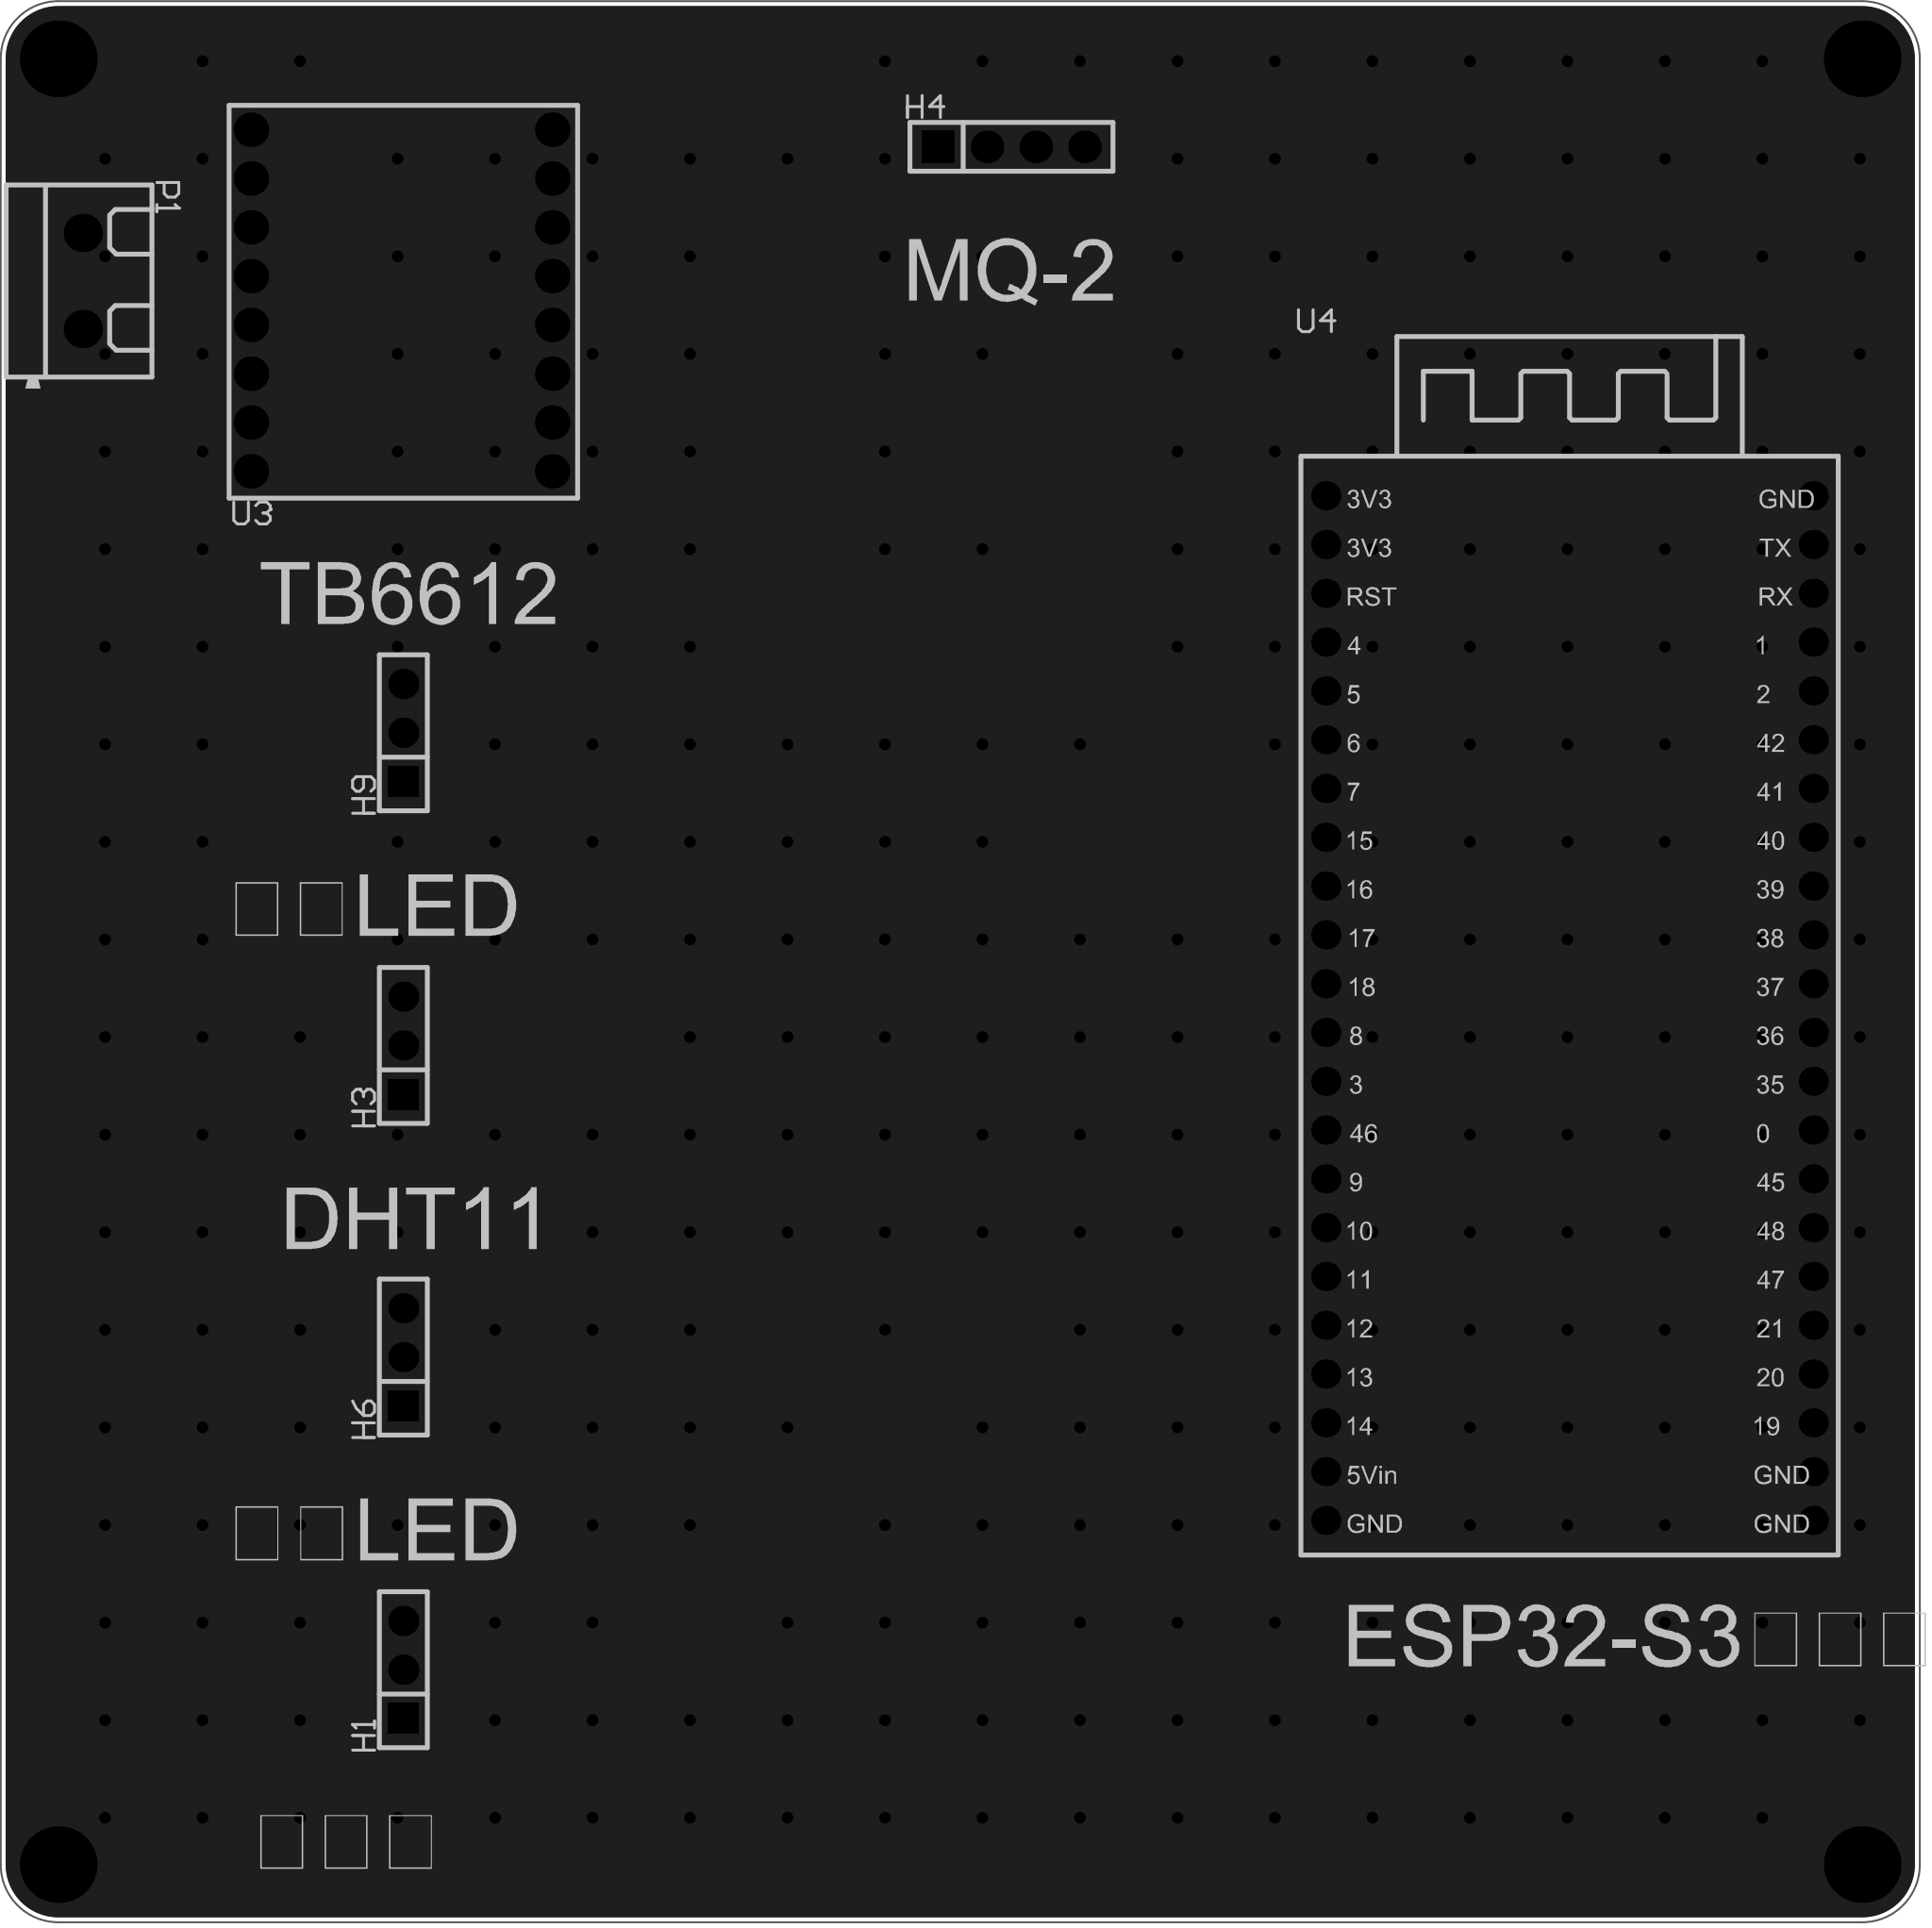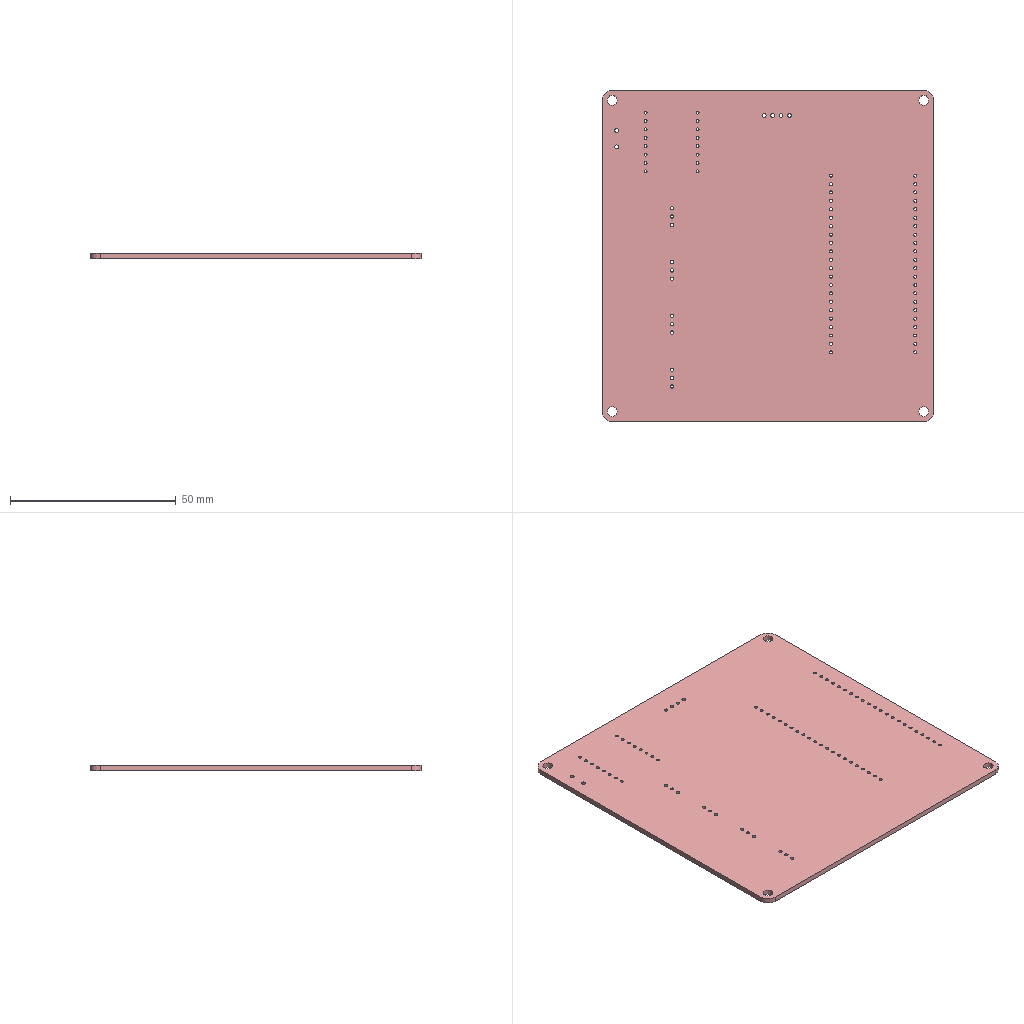Circuit board layout | Altium Designer | box 100 x 100 x 1.6 mm
Layer stack:
# Altium Designer layer stack of  (unit mm; dielectric type: 0 none, 1 core, 2 prepreg, 3 surface material)
index,name,kind,layer,copper_thickness_mm,dielectric_type,dielectric_thickness_mm,dielectric_material,dielectric_constant
0,Top Paste Mask Layer,other,,,,,,
1,Top Silkscreen Layer,other,,,,,,
2,Top Solder Mask Layer,dielectric,,,3,0.01,,3.3
3,Top Layer,copper,Top Layer,0.035,,,,
4,Dielectric1,dielectric,,,3,1.51,FR4,4.5
5,Bottom Layer,copper,Bottom Layer,0.035,,,,
6,Bottom Solder Mask Layer,dielectric,,,3,0.01,,3.3
7,Bottom Silkscreen Layer,other,,,,,,
8,Bottom Paste Mask Layer,other,,,,,,
# drill layer pairs: low layer,high layer
drill_pair,Top Layer,Bottom Layer
Part placement:
Designator,Comment,Layer,Footprint,Center-X(mm),Center-Y(mm),Rotation
H1,,TopLayer,HDR-TH_3P-P2.54-V-F,112.332,94.082,90
H3,,TopLayer,HDR-TH_3P-P2.54-V-F,112.332,126.578,90
H4,,TopLayer,HDR-TH_4P-P2.54-V-F,144.018,173.355,0
H6,,TopLayer,HDR-TH_3P-P2.54-V-F,112.332,110.357,90
H9,,TopLayer,HDR-TH_3P-P2.54-V-F,112.332,142.853,90
P1,KF301-2P接线端子,TopLayer,CONN-TH_XY301V-A-5.0-2P,95.631,166.37,270
U3,,TopLayer,tb6612,112.243,165.354,0
U4,NO,TopLayer,ESP32S3,173.101,128.524,0
Pad and via stacks:
# Altium Designer via and pad stacks of  (unit mm). Each distinct definition once, with the count of objects using it.
# via: kind,start_layer,end_layer,hole_mm,diameter_mm,mode(0 simple;1 top-mid-bottom;2 full stack),diameter_per_layer,count,example_net
# pad: kind,layer,hole_mm,hole_type(0 round;1 square;2 slot),plating,top_size,top_shape(1 round;2 rect;3 octagon;9 rounded rect),mid_size,bottom_size,mode,footprint,size_per_layer,count,example
pad,Multi-Layer,3,0,plated,4x4,1,4x4,4x4,0,,,4,1
pad,Multi-Layer,1.02,0,plated,1.575x1.575,1,1.575x1.575,1.575x1.575,0,HDR-TH_3P-P2.54-V-F,,8,H1.3
pad,Multi-Layer,1.02,0,plated,1.575x1.575,2,1.575x1.575,1.575x1.575,0,HDR-TH_3P-P2.54-V-F,,4,H1.1
pad,Multi-Layer,1.1,0,plated,1.7x1.7,2,1.7x1.7,1.7x1.7,0,HDR-TH_4P-P2.54-V-F,,1,H4.1
pad,Multi-Layer,1.1,0,plated,1.7x1.7,1,1.7x1.7,1.7x1.7,0,HDR-TH_4P-P2.54-V-F,,3,H4.2
pad,Multi-Layer,1.2,0,plated,2x2,1,2x2,2x2,0,CONN-TH_XY301V-A-5.0-2P,,2,P1.1
pad,Multi-Layer,0.9,0,plated,1.8x1.8,1,1.8x1.8,1.8x1.8,0,tb6612,,16,U3.1
pad,Multi-Layer,0.9144,0,plated,1.524x1.524,1,1.524x1.524,1.524x1.524,0,ESP32S3,,44,U4.1
via,Top Layer,Bottom Layer,0.3048,0.61,0,,311,GND
Copper pours:
name,layer,net,type(0 solid;1 hatched;2 none)
Bottom Layer-GND,Bottom Layer,GND,0
Top Layer-GND,Top Layer,GND,0
Design rules, without the lines most boards share:
# Altium Designer design rules of  (exported by Altium Designer, unit mm)
# columns: name | kind | enabled | priority | scope1 | scope2 | descriptor | typed fields (field=value)
Copper_copperRegion_copperThickness1oz | 0 | disabled | 4 | All | All | Clearance Constraint (Gap=5.984mil) (Disabled)(All),(All) | gap=0.152
Copper_copperRegion_copperThickness1oz_1 | 63 | disabled | 4 | All | All | Board Clearance Constraint (Gap=0mil) (Disabled)(All) |
Copper_copperRegion_Copper_copperRegion | 0 | disabled | 5 | All | All | Clearance Constraint (Gap=5.984mil) (Disabled)(All),(All) | gap=0.152
Copper_copperRegion_Copper_copperRegion_1 | 63 | disabled | 5 | All | All | Board Clearance Constraint (Gap=0mil) (Disabled)(All) |
copperThickness1oz | 0 | enabled | 6 | All | All | Clearance Constraint (Gap=5.984mil) (All),(All) | gap=0.152
copperThickness1oz_1 | 63 | enabled | 6 | All | All | Board Clearance Constraint (Gap=0mil) (All) |
copperRegion_copperThickness1oz | 20 | disabled | 1 | All | All | Polygon Connect Rule(Relief Connect )(Conductor Width=10mil) (Relief Angle=90 Angle) (Entries=4) (Air Gap Width=10mil) (Disabled)(All),(All) | connect_style(0=relief,1=direct,2=none)=0 relief_conductor_width=0.254 relief_entries=4
copperRegion_Copper_copperRegion | 20 | disabled | 2 | All | All | Polygon Connect Rule(Relief Connect )(Conductor Width=10mil) (Relief Angle=90 Angle) (Entries=4) (Air Gap Width=10mil) (Disabled)(All),(All) | connect_style(0=relief,1=direct,2=none)=0 relief_conductor_width=0.254 relief_entries=4
copperRegion | 20 | enabled | 3 | All | All | Polygon Connect Rule(Relief Connect )(Conductor Width=10mil) (Relief Angle=90 Angle) (Entries=4) (Air Gap Width=10mil) (All),(All) | connect_style(0=relief,1=direct,2=none)=0 relief_conductor_width=0.254 relief_entries=4